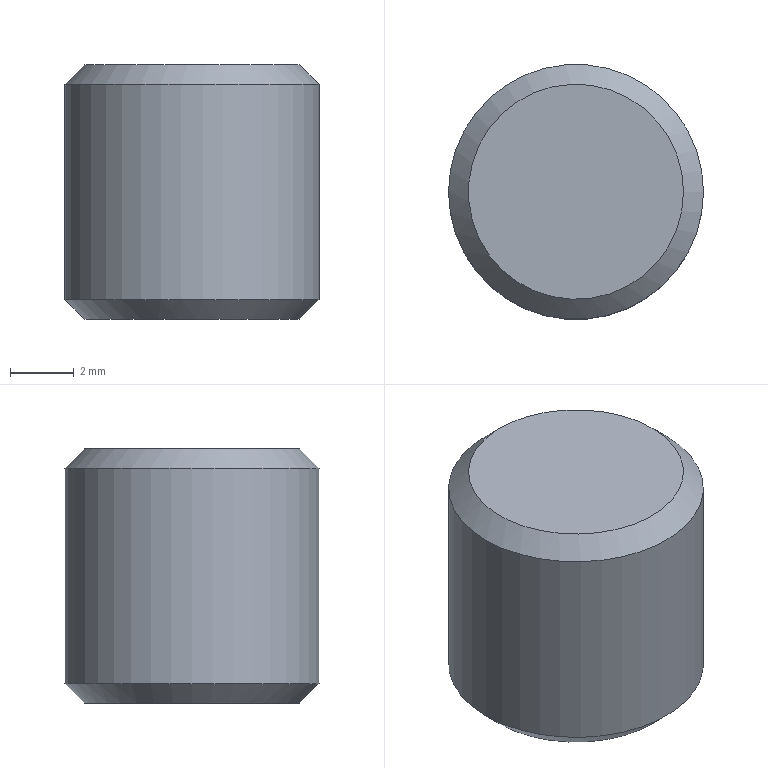Part | NX | features PG_666 2 | 1 solid | 5 faces | box 8 x 8 x 8 mm | volume 392.818 mm3 | plane 2 | cone 2 | cylinder 1 | commonest cylinder face diameters 8 x1
STEP:
#1=CARTESIAN_POINT('',(3520.62,-821.296,789.716));
#2=VERTEX_POINT('',#1);
#3=CARTESIAN_POINT('',(3523.995,-821.296,789.716));
#4=DIRECTION('',(0.,0.,1.));
#5=DIRECTION('',(-1.,0.,0.));
#6=AXIS2_PLACEMENT_3D('',#3,#4,#5);
#7=CIRCLE('',#6,3.375);
#8=EDGE_CURVE('',#2,#2,#7,.T.);
#9=ORIENTED_EDGE('',*,*,#8,.F.);
#10=EDGE_LOOP('',(#9));
#11=FACE_BOUND('',#10,.T.);
#12=CARTESIAN_POINT('',(3523.995,-821.296,789.716));
#13=DIRECTION('',(0.,0.,-1.));
#14=DIRECTION('',(-1.,0.,0.));
#15=AXIS2_PLACEMENT_3D('',#12,#13,#14);
#16=PLANE('',#15);
#17=ADVANCED_FACE('',(#11),#16,.T.);
#18=CARTESIAN_POINT('',(3527.37,-821.296,797.716));
#19=VERTEX_POINT('',#18);
#20=CARTESIAN_POINT('',(3523.995,-821.296,797.716));
#21=DIRECTION('',(0.,0.,-1.));
#22=DIRECTION('',(1.,0.,0.));
#23=AXIS2_PLACEMENT_3D('',#20,#21,#22);
#24=CIRCLE('',#23,3.375);
#25=EDGE_CURVE('',#19,#19,#24,.T.);
#26=ORIENTED_EDGE('',*,*,#25,.F.);
#27=EDGE_LOOP('',(#26));
#28=FACE_BOUND('',#27,.T.);
#29=CARTESIAN_POINT('',(3523.995,-821.296,797.716));
#30=DIRECTION('',(0.,0.,1.));
#31=DIRECTION('',(1.,0.,0.));
#32=AXIS2_PLACEMENT_3D('',#29,#30,#31);
#33=PLANE('',#32);
#34=ADVANCED_FACE('',(#28),#33,.T.);
#35=CARTESIAN_POINT('',(3527.995,-821.296,797.091));
#36=VERTEX_POINT('',#35);
#37=CARTESIAN_POINT('',(3523.995,-821.296,797.091));
#38=DIRECTION('',(0.,0.,-1.));
#39=DIRECTION('',(1.,0.,0.));
#40=AXIS2_PLACEMENT_3D('',#37,#38,#39);
#41=CIRCLE('',#40,4.);
#42=EDGE_CURVE('',#36,#36,#41,.F.);
#43=ORIENTED_EDGE('',*,*,#42,.F.);
#44=EDGE_LOOP('',(#43));
#45=FACE_BOUND('',#44,.T.);
#46=CARTESIAN_POINT('',(3519.995,-821.296,790.341));
#47=VERTEX_POINT('',#46);
#48=CARTESIAN_POINT('',(3523.995,-821.296,790.341));
#49=DIRECTION('',(0.,0.,1.));
#50=DIRECTION('',(-1.,0.,0.));
#51=AXIS2_PLACEMENT_3D('',#48,#49,#50);
#52=CIRCLE('',#51,4.);
#53=EDGE_CURVE('',#47,#47,#52,.F.);
#54=ORIENTED_EDGE('',*,*,#53,.F.);
#55=EDGE_LOOP('',(#54));
#56=FACE_BOUND('',#55,.T.);
#57=CARTESIAN_POINT('',(3523.995,-821.296,858.716));
#58=DIRECTION('',(0.,0.,-1.));
#59=DIRECTION('',(-1.,0.,0.));
#60=AXIS2_PLACEMENT_3D('',#57,#58,#59);
#61=CYLINDRICAL_SURFACE('',#60,4.);
#62=ADVANCED_FACE('',(#45,#56),#61,.T.);
#63=ORIENTED_EDGE('',*,*,#25,.T.);
#64=EDGE_LOOP('',(#63));
#65=FACE_BOUND('',#64,.T.);
#66=ORIENTED_EDGE('',*,*,#42,.T.);
#67=EDGE_LOOP('',(#66));
#68=FACE_BOUND('',#67,.T.);
#69=CARTESIAN_POINT('',(3523.995,-821.296,797.091));
#70=DIRECTION('',(0.,0.,-1.));
#71=DIRECTION('',(-1.,0.,0.));
#72=AXIS2_PLACEMENT_3D('',#69,#70,#71);
#73=CONICAL_SURFACE('',#72,4.,0.7854);
#74=ADVANCED_FACE('',(#65,#68),#73,.T.);
#75=ORIENTED_EDGE('',*,*,#8,.T.);
#76=EDGE_LOOP('',(#75));
#77=FACE_BOUND('',#76,.T.);
#78=ORIENTED_EDGE('',*,*,#53,.T.);
#79=EDGE_LOOP('',(#78));
#80=FACE_BOUND('',#79,.T.);
#81=CARTESIAN_POINT('',(3523.995,-821.296,790.341));
#82=DIRECTION('',(0.,0.,1.));
#83=DIRECTION('',(1.,0.,0.));
#84=AXIS2_PLACEMENT_3D('',#81,#82,#83);
#85=CONICAL_SURFACE('',#84,4.,0.7854);
#86=ADVANCED_FACE('',(#77,#80),#85,.T.);
#87=CLOSED_SHELL('',(#17,#34,#62,#74,#86));
#88=MANIFOLD_SOLID_BREP('',#87);
#89=(LENGTH_UNIT()NAMED_UNIT(*)SI_UNIT(.MILLI.,.METRE.));
#90=UNCERTAINTY_MEASURE_WITH_UNIT(LENGTH_MEASURE(0.00001),#89,'','');
#91=(NAMED_UNIT(*)PLANE_ANGLE_UNIT()SI_UNIT($,.RADIAN.));
#92=(NAMED_UNIT(*)SI_UNIT($,.STERADIAN.)SOLID_ANGLE_UNIT());
#93=(GEOMETRIC_REPRESENTATION_CONTEXT(3)GLOBAL_UNCERTAINTY_ASSIGNED_CONTEXT((#90))GLOBAL_UNIT_ASSIGNED_CONTEXT((#89,#91,#92))REPRESENTATION_CONTEXT('',''));
#94=ADVANCED_BREP_SHAPE_REPRESENTATION('',(#88),#93);